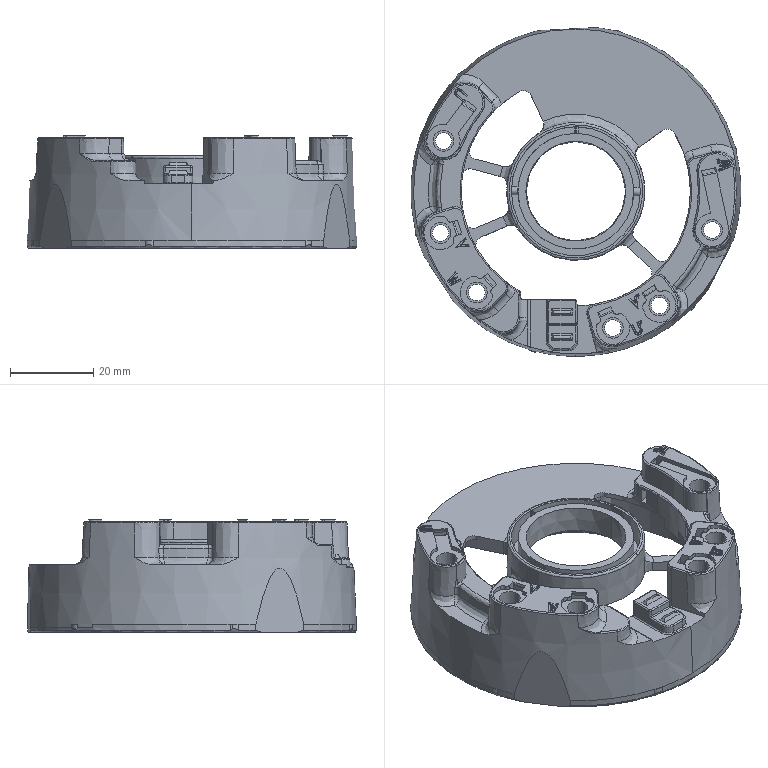Part | STEP file | TQ-DD-1105-THA160078900_Mold1010_デフォルト | 1 solid | 900 faces | box 79.236 x 78.917 x 27.1 mm | volume 21027 mm3 | cylinder 390 | plane 335 | spline 144 | cone 31 | commonest cylinder face diameters 0.2 x68 0.6 x63 2 x58 4 x51 5 x24 3.6 x18